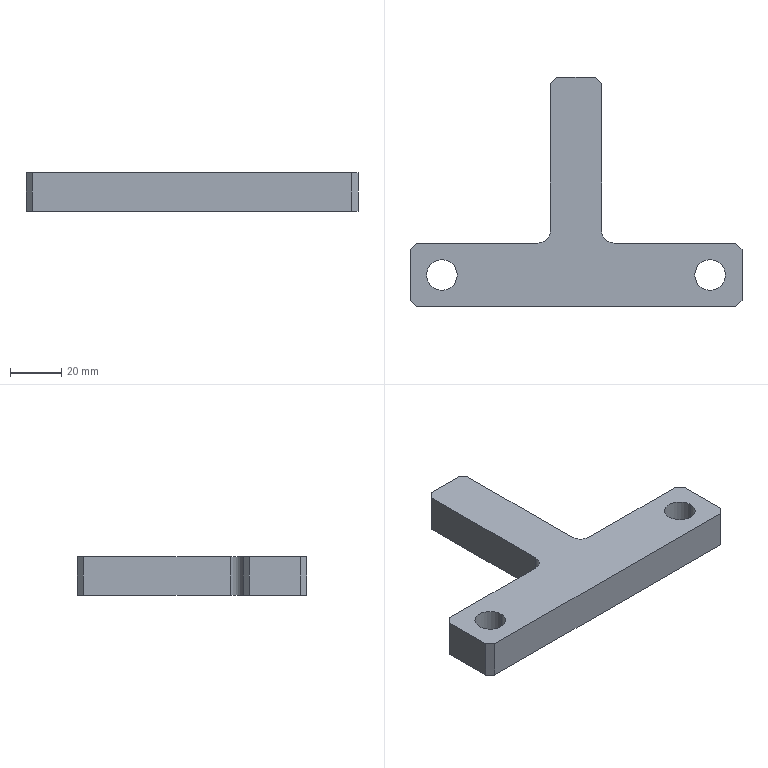Part | STEP file | Polisher shift lever | 1 solid | 22 faces | box 130 x 90 x 15 mm | volume 64737 mm3 | plane 16 | cylinder 6 | commonest cylinder face diameters 12 x4 10 x2